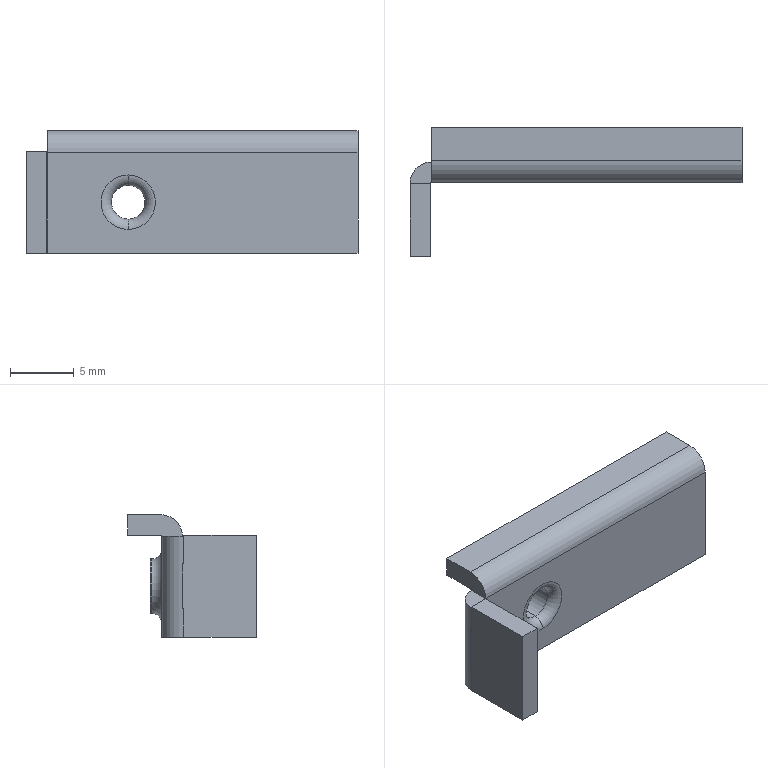Part | STEP file | LRS-150-12_X2_5F00517375-151316 | 1 solid | 27 faces | box 26 x 10.1 x 9.6 mm | volume 553.854 mm3 | plane 15 | cylinder 8 | torus 4 | commonest cylinder face diameters 0.2 x2 2.65 x2 3.4 x2 4.27 x2